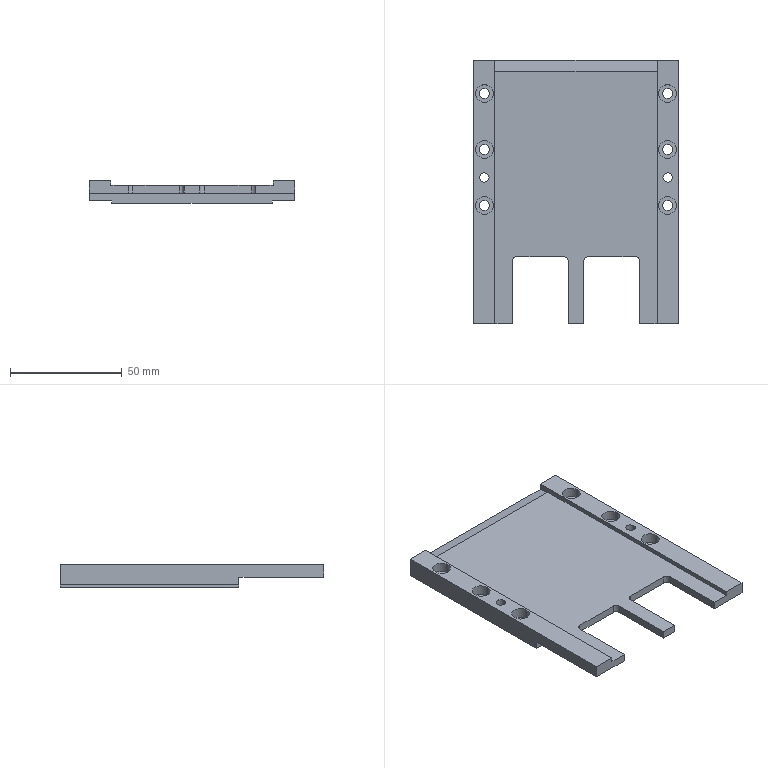Part | STEP file | 2021 Bottom plate | 1 solid | 63 faces | box 92 x 118 x 10 mm | volume 66642 mm3 | cylinder 32 | plane 31 | commonest cylinder face diameters 4.5 x12 8 x12 4 x4 4.2 x4